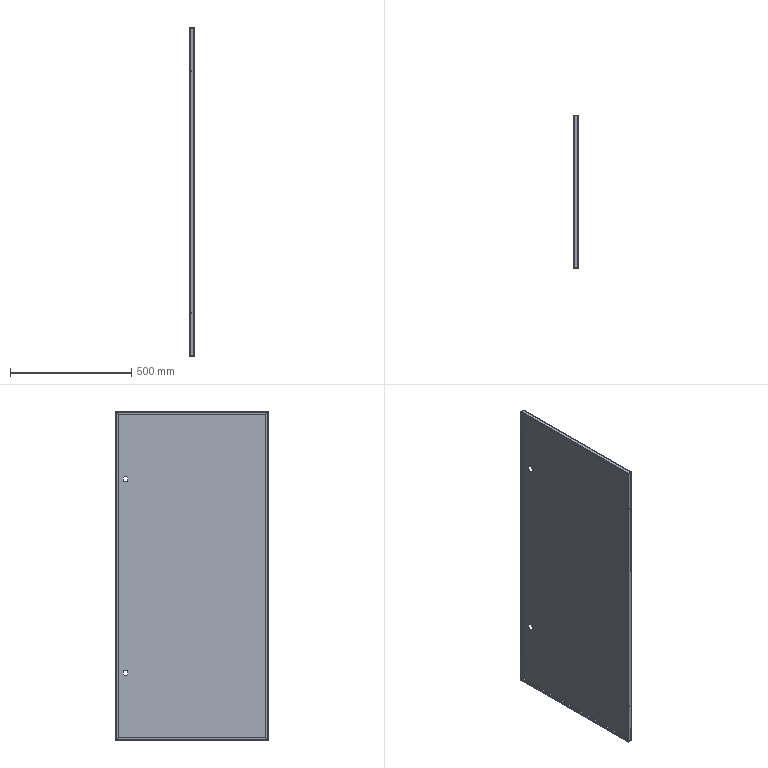Part | STEP file | HESS-408-70-15W-W-19-side door panel | 1 solid | 106 faces | box 18 x 629 x 1358 mm | volume 1424005 mm3 | plane 70 | cylinder 28 | spline 8 | commonest cylinder face diameters 0.2 x8 3.2 x8 22.5 x8 5 x4